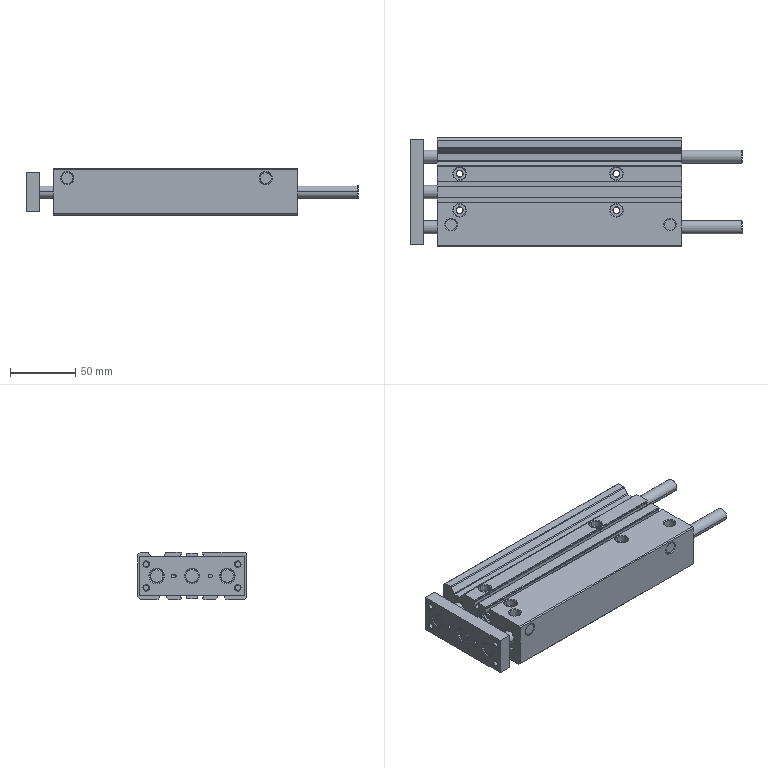Part | SolidWorks | 2 solids | 389 faces | box 254 x 83 x 36 mm | volume 461656 mm3 | cylinder 173 | plane 120 | cone 94 | spline 2 | commonest cylinder face diameters 3 x21 0.8 x20 4.134 x16 10 x16 0.4 x12 0.6 x10